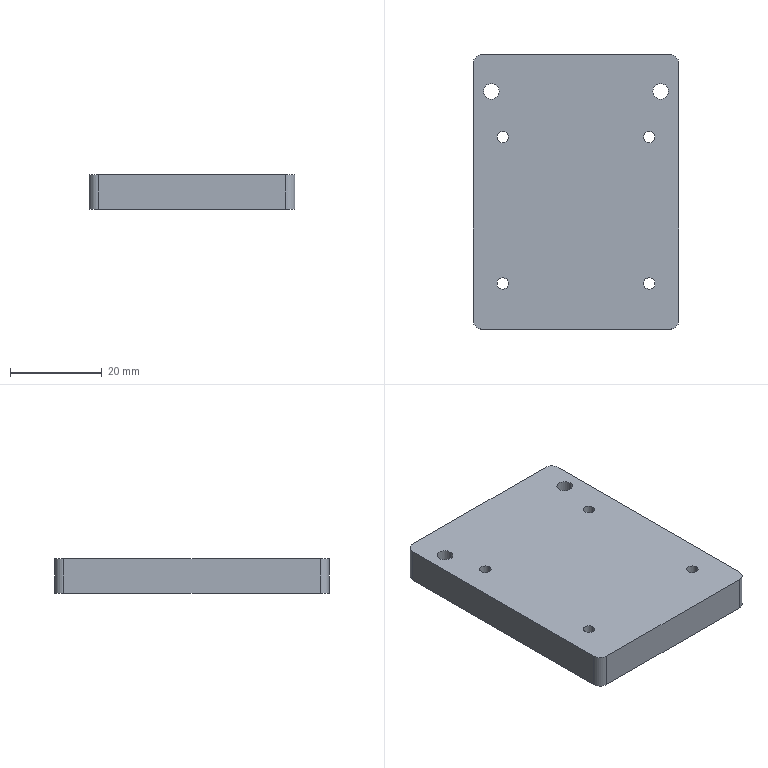Part | STEP file | Guide wheel mechanism revised.sldasm-Part-47 | 1 solid | 28 faces | box 45 x 60 x 7.6 mm | volume 20043 mm3 | cylinder 20 | plane 8 | commonest cylinder face diameters 2.5 x8 3.4 x4 4 x4 6.5 x4
STEP:
#1=CARTESIAN_POINT('',(-15.25,22.,-0.4));
#2=VERTEX_POINT('',#1);
#3=CARTESIAN_POINT('',(-21.75,22.,-0.4));
#4=VERTEX_POINT('',#3);
#5=CARTESIAN_POINT('',(-18.5,22.,-0.4));
#6=DIRECTION('',(0.,0.,-1.));
#7=DIRECTION('',(-1.,0.,0.));
#8=AXIS2_PLACEMENT_3D('',#5,#6,#7);
#9=CIRCLE('',#8,3.25);
#10=EDGE_CURVE('',#2,#4,#9,.T.);
#11=ORIENTED_EDGE('',*,*,#10,.F.);
#12=CARTESIAN_POINT('',(-15.25,22.,-3.8));
#13=VERTEX_POINT('',#12);
#14=CARTESIAN_POINT('',(-15.25,22.,-3.8));
#15=DIRECTION('',(0.,0.,-1.));
#16=VECTOR('',#15,1000.);
#17=LINE('',#14,#16);
#18=EDGE_CURVE('',#2,#13,#17,.T.);
#19=ORIENTED_EDGE('',*,*,#18,.T.);
#20=CARTESIAN_POINT('',(-21.75,22.,-3.8));
#21=VERTEX_POINT('',#20);
#22=CARTESIAN_POINT('',(-18.5,22.,-3.8));
#23=DIRECTION('',(0.,0.,-1.));
#24=DIRECTION('',(-1.,0.,0.));
#25=AXIS2_PLACEMENT_3D('',#22,#23,#24);
#26=CIRCLE('',#25,3.25);
#27=EDGE_CURVE('',#13,#21,#26,.T.);
#28=ORIENTED_EDGE('',*,*,#27,.T.);
#29=CARTESIAN_POINT('',(-21.75,22.,-3.8));
#30=DIRECTION('',(0.,0.,-1.));
#31=VECTOR('',#30,1000.);
#32=LINE('',#29,#31);
#33=EDGE_CURVE('',#4,#21,#32,.T.);
#34=ORIENTED_EDGE('',*,*,#33,.F.);
#35=EDGE_LOOP('',(#11,#19,#28,#34));
#36=FACE_OUTER_BOUND('',#35,.T.);
#37=CARTESIAN_POINT('',(-18.5,22.,-3.8));
#38=DIRECTION('',(0.,0.,-1.));
#39=DIRECTION('',(-1.,0.,0.));
#40=AXIS2_PLACEMENT_3D('',#37,#38,#39);
#41=CYLINDRICAL_SURFACE('',#40,3.25);
#42=ADVANCED_FACE('',(#36),#41,.F.);
#43=CARTESIAN_POINT('',(-16.8,22.,3.8));
#44=VERTEX_POINT('',#43);
#45=CARTESIAN_POINT('',(-20.2,22.,3.8));
#46=VERTEX_POINT('',#45);
#47=CARTESIAN_POINT('',(-18.5,22.,3.8));
#48=DIRECTION('',(0.,0.,-1.));
#49=DIRECTION('',(-1.,0.,0.));
#50=AXIS2_PLACEMENT_3D('',#47,#48,#49);
#51=CIRCLE('',#50,1.7);
#52=EDGE_CURVE('',#44,#46,#51,.T.);
#53=ORIENTED_EDGE('',*,*,#52,.F.);
#54=CARTESIAN_POINT('',(-16.8,22.,-0.4));
#55=VERTEX_POINT('',#54);
#56=CARTESIAN_POINT('',(-16.8,22.,-3.8));
#57=DIRECTION('',(0.,0.,-1.));
#58=VECTOR('',#57,1000.);
#59=LINE('',#56,#58);
#60=EDGE_CURVE('',#44,#55,#59,.T.);
#61=ORIENTED_EDGE('',*,*,#60,.T.);
#62=CARTESIAN_POINT('',(-20.2,22.,-0.4));
#63=VERTEX_POINT('',#62);
#64=CARTESIAN_POINT('',(-18.5,22.,-0.4));
#65=DIRECTION('',(0.,0.,-1.));
#66=DIRECTION('',(-1.,0.,0.));
#67=AXIS2_PLACEMENT_3D('',#64,#65,#66);
#68=CIRCLE('',#67,1.7);
#69=EDGE_CURVE('',#55,#63,#68,.T.);
#70=ORIENTED_EDGE('',*,*,#69,.T.);
#71=CARTESIAN_POINT('',(-20.2,22.,-3.8));
#72=DIRECTION('',(0.,0.,-1.));
#73=VECTOR('',#72,1000.);
#74=LINE('',#71,#73);
#75=EDGE_CURVE('',#46,#63,#74,.T.);
#76=ORIENTED_EDGE('',*,*,#75,.F.);
#77=EDGE_LOOP('',(#53,#61,#70,#76));
#78=FACE_OUTER_BOUND('',#77,.T.);
#79=CARTESIAN_POINT('',(-18.5,22.,-3.8));
#80=DIRECTION('',(0.,0.,-1.));
#81=DIRECTION('',(-1.,0.,0.));
#82=AXIS2_PLACEMENT_3D('',#79,#80,#81);
#83=CYLINDRICAL_SURFACE('',#82,1.7);
#84=ADVANCED_FACE('',(#78),#83,.F.);
#85=CARTESIAN_POINT('',(21.75,22.,-0.4));
#86=VERTEX_POINT('',#85);
#87=CARTESIAN_POINT('',(15.25,22.,-0.4));
#88=VERTEX_POINT('',#87);
#89=CARTESIAN_POINT('',(18.5,22.,-0.4));
#90=DIRECTION('',(0.,0.,-1.));
#91=DIRECTION('',(-1.,0.,0.));
#92=AXIS2_PLACEMENT_3D('',#89,#90,#91);
#93=CIRCLE('',#92,3.25);
#94=EDGE_CURVE('',#86,#88,#93,.T.);
#95=ORIENTED_EDGE('',*,*,#94,.F.);
#96=CARTESIAN_POINT('',(21.75,22.,-3.8));
#97=VERTEX_POINT('',#96);
#98=CARTESIAN_POINT('',(21.75,22.,-3.8));
#99=DIRECTION('',(0.,0.,-1.));
#100=VECTOR('',#99,1000.);
#101=LINE('',#98,#100);
#102=EDGE_CURVE('',#86,#97,#101,.T.);
#103=ORIENTED_EDGE('',*,*,#102,.T.);
#104=CARTESIAN_POINT('',(15.25,22.,-3.8));
#105=VERTEX_POINT('',#104);
#106=CARTESIAN_POINT('',(18.5,22.,-3.8));
#107=DIRECTION('',(0.,0.,-1.));
#108=DIRECTION('',(-1.,0.,0.));
#109=AXIS2_PLACEMENT_3D('',#106,#107,#108);
#110=CIRCLE('',#109,3.25);
#111=EDGE_CURVE('',#97,#105,#110,.T.);
#112=ORIENTED_EDGE('',*,*,#111,.T.);
#113=CARTESIAN_POINT('',(15.25,22.,-3.8));
#114=DIRECTION('',(0.,0.,-1.));
#115=VECTOR('',#114,1000.);
#116=LINE('',#113,#115);
#117=EDGE_CURVE('',#88,#105,#116,.T.);
#118=ORIENTED_EDGE('',*,*,#117,.F.);
#119=EDGE_LOOP('',(#95,#103,#112,#118));
#120=FACE_OUTER_BOUND('',#119,.T.);
#121=CARTESIAN_POINT('',(18.5,22.,-3.8));
#122=DIRECTION('',(0.,0.,-1.));
#123=DIRECTION('',(-1.,0.,0.));
#124=AXIS2_PLACEMENT_3D('',#121,#122,#123);
#125=CYLINDRICAL_SURFACE('',#124,3.25);
#126=ADVANCED_FACE('',(#120),#125,.F.);
#127=CARTESIAN_POINT('',(20.2,22.,3.8));
#128=VERTEX_POINT('',#127);
#129=CARTESIAN_POINT('',(16.8,22.,3.8));
#130=VERTEX_POINT('',#129);
#131=CARTESIAN_POINT('',(18.5,22.,3.8));
#132=DIRECTION('',(0.,0.,-1.));
#133=DIRECTION('',(-1.,0.,0.));
#134=AXIS2_PLACEMENT_3D('',#131,#132,#133);
#135=CIRCLE('',#134,1.7);
#136=EDGE_CURVE('',#128,#130,#135,.T.);
#137=ORIENTED_EDGE('',*,*,#136,.F.);
#138=CARTESIAN_POINT('',(20.2,22.,-0.4));
#139=VERTEX_POINT('',#138);
#140=CARTESIAN_POINT('',(20.2,22.,-3.8));
#141=DIRECTION('',(0.,0.,-1.));
#142=VECTOR('',#141,1000.);
#143=LINE('',#140,#142);
#144=EDGE_CURVE('',#128,#139,#143,.T.);
#145=ORIENTED_EDGE('',*,*,#144,.T.);
#146=CARTESIAN_POINT('',(16.8,22.,-0.4));
#147=VERTEX_POINT('',#146);
#148=CARTESIAN_POINT('',(18.5,22.,-0.4));
#149=DIRECTION('',(0.,0.,-1.));
#150=DIRECTION('',(-1.,0.,0.));
#151=AXIS2_PLACEMENT_3D('',#148,#149,#150);
#152=CIRCLE('',#151,1.7);
#153=EDGE_CURVE('',#139,#147,#152,.T.);
#154=ORIENTED_EDGE('',*,*,#153,.T.);
#155=CARTESIAN_POINT('',(16.8,22.,-3.8));
#156=DIRECTION('',(0.,0.,-1.));
#157=VECTOR('',#156,1000.);
#158=LINE('',#155,#157);
#159=EDGE_CURVE('',#130,#147,#158,.T.);
#160=ORIENTED_EDGE('',*,*,#159,.F.);
#161=EDGE_LOOP('',(#137,#145,#154,#160));
#162=FACE_OUTER_BOUND('',#161,.T.);
#163=CARTESIAN_POINT('',(18.5,22.,-3.8));
#164=DIRECTION('',(0.,0.,-1.));
#165=DIRECTION('',(-1.,0.,0.));
#166=AXIS2_PLACEMENT_3D('',#163,#164,#165);
#167=CYLINDRICAL_SURFACE('',#166,1.7);
#168=ADVANCED_FACE('',(#162),#167,.F.);
#169=CARTESIAN_POINT('',(14.75,12.,-3.8));
#170=VERTEX_POINT('',#169);
#171=CARTESIAN_POINT('',(17.25,12.,-3.8));
#172=VERTEX_POINT('',#171);
#173=CARTESIAN_POINT('',(16.,12.,-3.8));
#174=DIRECTION('',(0.,0.,1.));
#175=DIRECTION('',(1.,0.,0.));
#176=AXIS2_PLACEMENT_3D('',#173,#174,#175);
#177=CIRCLE('',#176,1.25);
#178=EDGE_CURVE('',#170,#172,#177,.T.);
#179=ORIENTED_EDGE('',*,*,#178,.F.);
#180=CARTESIAN_POINT('',(14.75,12.,3.8));
#181=VERTEX_POINT('',#180);
#182=CARTESIAN_POINT('',(14.75,12.,3.8));
#183=DIRECTION('',(0.,0.,1.));
#184=VECTOR('',#183,1000.);
#185=LINE('',#182,#184);
#186=EDGE_CURVE('',#170,#181,#185,.T.);
#187=ORIENTED_EDGE('',*,*,#186,.T.);
#188=CARTESIAN_POINT('',(17.25,12.,3.8));
#189=VERTEX_POINT('',#188);
#190=CARTESIAN_POINT('',(16.,12.,3.8));
#191=DIRECTION('',(0.,0.,1.));
#192=DIRECTION('',(1.,0.,0.));
#193=AXIS2_PLACEMENT_3D('',#190,#191,#192);
#194=CIRCLE('',#193,1.25);
#195=EDGE_CURVE('',#181,#189,#194,.T.);
#196=ORIENTED_EDGE('',*,*,#195,.T.);
#197=CARTESIAN_POINT('',(17.25,12.,3.8));
#198=DIRECTION('',(0.,0.,1.));
#199=VECTOR('',#198,1000.);
#200=LINE('',#197,#199);
#201=EDGE_CURVE('',#172,#189,#200,.T.);
#202=ORIENTED_EDGE('',*,*,#201,.F.);
#203=EDGE_LOOP('',(#179,#187,#196,#202));
#204=FACE_OUTER_BOUND('',#203,.T.);
#205=CARTESIAN_POINT('',(16.,12.,3.8));
#206=DIRECTION('',(0.,0.,1.));
#207=DIRECTION('',(1.,0.,0.));
#208=AXIS2_PLACEMENT_3D('',#205,#206,#207);
#209=CYLINDRICAL_SURFACE('',#208,1.25);
#210=ADVANCED_FACE('',(#204),#209,.F.);
#211=CARTESIAN_POINT('',(-17.25,12.,-3.8));
#212=VERTEX_POINT('',#211);
#213=CARTESIAN_POINT('',(-14.75,12.,-3.8));
#214=VERTEX_POINT('',#213);
#215=CARTESIAN_POINT('',(-16.,12.,-3.8));
#216=DIRECTION('',(0.,0.,1.));
#217=DIRECTION('',(1.,0.,0.));
#218=AXIS2_PLACEMENT_3D('',#215,#216,#217);
#219=CIRCLE('',#218,1.25);
#220=EDGE_CURVE('',#212,#214,#219,.T.);
#221=ORIENTED_EDGE('',*,*,#220,.F.);
#222=CARTESIAN_POINT('',(-17.25,12.,3.8));
#223=VERTEX_POINT('',#222);
#224=CARTESIAN_POINT('',(-17.25,12.,3.8));
#225=DIRECTION('',(0.,0.,1.));
#226=VECTOR('',#225,1000.);
#227=LINE('',#224,#226);
#228=EDGE_CURVE('',#212,#223,#227,.T.);
#229=ORIENTED_EDGE('',*,*,#228,.T.);
#230=CARTESIAN_POINT('',(-14.75,12.,3.8));
#231=VERTEX_POINT('',#230);
#232=CARTESIAN_POINT('',(-16.,12.,3.8));
#233=DIRECTION('',(0.,0.,1.));
#234=DIRECTION('',(1.,0.,0.));
#235=AXIS2_PLACEMENT_3D('',#232,#233,#234);
#236=CIRCLE('',#235,1.25);
#237=EDGE_CURVE('',#223,#231,#236,.T.);
#238=ORIENTED_EDGE('',*,*,#237,.T.);
#239=CARTESIAN_POINT('',(-14.75,12.,3.8));
#240=DIRECTION('',(0.,0.,1.));
#241=VECTOR('',#240,1000.);
#242=LINE('',#239,#241);
#243=EDGE_CURVE('',#214,#231,#242,.T.);
#244=ORIENTED_EDGE('',*,*,#243,.F.);
#245=EDGE_LOOP('',(#221,#229,#238,#244));
#246=FACE_OUTER_BOUND('',#245,.T.);
#247=CARTESIAN_POINT('',(-16.,12.,3.8));
#248=DIRECTION('',(0.,0.,1.));
#249=DIRECTION('',(1.,0.,0.));
#250=AXIS2_PLACEMENT_3D('',#247,#248,#249);
#251=CYLINDRICAL_SURFACE('',#250,1.25);
#252=ADVANCED_FACE('',(#246),#251,.F.);
#253=CARTESIAN_POINT('',(-17.25,-20.,-3.8));
#254=VERTEX_POINT('',#253);
#255=CARTESIAN_POINT('',(-14.75,-20.,-3.8));
#256=VERTEX_POINT('',#255);
#257=CARTESIAN_POINT('',(-16.,-20.,-3.8));
#258=DIRECTION('',(0.,0.,1.));
#259=DIRECTION('',(1.,0.,0.));
#260=AXIS2_PLACEMENT_3D('',#257,#258,#259);
#261=CIRCLE('',#260,1.25);
#262=EDGE_CURVE('',#254,#256,#261,.T.);
#263=ORIENTED_EDGE('',*,*,#262,.F.);
#264=CARTESIAN_POINT('',(-17.25,-20.,3.8));
#265=VERTEX_POINT('',#264);
#266=CARTESIAN_POINT('',(-17.25,-20.,3.8));
#267=DIRECTION('',(0.,0.,1.));
#268=VECTOR('',#267,1000.);
#269=LINE('',#266,#268);
#270=EDGE_CURVE('',#254,#265,#269,.T.);
#271=ORIENTED_EDGE('',*,*,#270,.T.);
#272=CARTESIAN_POINT('',(-14.75,-20.,3.8));
#273=VERTEX_POINT('',#272);
#274=CARTESIAN_POINT('',(-16.,-20.,3.8));
#275=DIRECTION('',(0.,0.,1.));
#276=DIRECTION('',(1.,0.,0.));
#277=AXIS2_PLACEMENT_3D('',#274,#275,#276);
#278=CIRCLE('',#277,1.25);
#279=EDGE_CURVE('',#265,#273,#278,.T.);
#280=ORIENTED_EDGE('',*,*,#279,.T.);
#281=CARTESIAN_POINT('',(-14.75,-20.,3.8));
#282=DIRECTION('',(0.,0.,1.));
#283=VECTOR('',#282,1000.);
#284=LINE('',#281,#283);
#285=EDGE_CURVE('',#256,#273,#284,.T.);
#286=ORIENTED_EDGE('',*,*,#285,.F.);
#287=EDGE_LOOP('',(#263,#271,#280,#286));
#288=FACE_OUTER_BOUND('',#287,.T.);
#289=CARTESIAN_POINT('',(-16.,-20.,3.8));
#290=DIRECTION('',(0.,0.,1.));
#291=DIRECTION('',(1.,0.,0.));
#292=AXIS2_PLACEMENT_3D('',#289,#290,#291);
#293=CYLINDRICAL_SURFACE('',#292,1.25);
#294=ADVANCED_FACE('',(#288),#293,.F.);
#295=CARTESIAN_POINT('',(14.75,-20.,-3.8));
#296=VERTEX_POINT('',#295);
#297=CARTESIAN_POINT('',(17.25,-20.,-3.8));
#298=VERTEX_POINT('',#297);
#299=CARTESIAN_POINT('',(16.,-20.,-3.8));
#300=DIRECTION('',(0.,0.,1.));
#301=DIRECTION('',(1.,0.,0.));
#302=AXIS2_PLACEMENT_3D('',#299,#300,#301);
#303=CIRCLE('',#302,1.25);
#304=EDGE_CURVE('',#296,#298,#303,.T.);
#305=ORIENTED_EDGE('',*,*,#304,.F.);
#306=CARTESIAN_POINT('',(14.75,-20.,3.8));
#307=VERTEX_POINT('',#306);
#308=CARTESIAN_POINT('',(14.75,-20.,3.8));
#309=DIRECTION('',(0.,0.,1.));
#310=VECTOR('',#309,1000.);
#311=LINE('',#308,#310);
#312=EDGE_CURVE('',#296,#307,#311,.T.);
#313=ORIENTED_EDGE('',*,*,#312,.T.);
#314=CARTESIAN_POINT('',(17.25,-20.,3.8));
#315=VERTEX_POINT('',#314);
#316=CARTESIAN_POINT('',(16.,-20.,3.8));
#317=DIRECTION('',(0.,0.,1.));
#318=DIRECTION('',(1.,0.,0.));
#319=AXIS2_PLACEMENT_3D('',#316,#317,#318);
#320=CIRCLE('',#319,1.25);
#321=EDGE_CURVE('',#307,#315,#320,.T.);
#322=ORIENTED_EDGE('',*,*,#321,.T.);
#323=CARTESIAN_POINT('',(17.25,-20.,3.8));
#324=DIRECTION('',(0.,0.,1.));
#325=VECTOR('',#324,1000.);
#326=LINE('',#323,#325);
#327=EDGE_CURVE('',#298,#315,#326,.T.);
#328=ORIENTED_EDGE('',*,*,#327,.F.);
#329=EDGE_LOOP('',(#305,#313,#322,#328));
#330=FACE_OUTER_BOUND('',#329,.T.);
#331=CARTESIAN_POINT('',(16.,-20.,3.8));
#332=DIRECTION('',(0.,0.,1.));
#333=DIRECTION('',(1.,0.,0.));
#334=AXIS2_PLACEMENT_3D('',#331,#332,#333);
#335=CYLINDRICAL_SURFACE('',#334,1.25);
#336=ADVANCED_FACE('',(#330),#335,.F.);
#337=CARTESIAN_POINT('',(22.5,-28.,3.8));
#338=VERTEX_POINT('',#337);
#339=CARTESIAN_POINT('',(22.5,28.,3.8));
#340=VERTEX_POINT('',#339);
#341=CARTESIAN_POINT('',(22.5,-30.,3.8));
#342=DIRECTION('',(0.,1.,0.));
#343=VECTOR('',#342,1000.);
#344=LINE('',#341,#343);
#345=EDGE_CURVE('',#338,#340,#344,.T.);
#346=ORIENTED_EDGE('',*,*,#345,.F.);
#347=CARTESIAN_POINT('',(22.5,-28.,-3.8));
#348=VERTEX_POINT('',#347);
#349=CARTESIAN_POINT('',(22.5,-28.,3.8));
#350=DIRECTION('',(0.,0.,-1.));
#351=VECTOR('',#350,1000.);
#352=LINE('',#349,#351);
#353=EDGE_CURVE('',#338,#348,#352,.T.);
#354=ORIENTED_EDGE('',*,*,#353,.T.);
#355=CARTESIAN_POINT('',(22.5,28.,-3.8));
#356=VERTEX_POINT('',#355);
#357=CARTESIAN_POINT('',(22.5,-30.,-3.8));
#358=DIRECTION('',(0.,1.,0.));
#359=VECTOR('',#358,1000.);
#360=LINE('',#357,#359);
#361=EDGE_CURVE('',#348,#356,#360,.T.);
#362=ORIENTED_EDGE('',*,*,#361,.T.);
#363=CARTESIAN_POINT('',(22.5,28.,3.8));
#364=DIRECTION('',(0.,0.,1.));
#365=VECTOR('',#364,1000.);
#366=LINE('',#363,#365);
#367=EDGE_CURVE('',#356,#340,#366,.T.);
#368=ORIENTED_EDGE('',*,*,#367,.T.);
#369=EDGE_LOOP('',(#346,#354,#362,#368));
#370=FACE_OUTER_BOUND('',#369,.T.);
#371=CARTESIAN_POINT('',(22.5,-30.,3.8));
#372=DIRECTION('',(-1.,0.,0.));
#373=DIRECTION('',(0.,0.,1.));
#374=AXIS2_PLACEMENT_3D('',#371,#372,#373);
#375=PLANE('',#374);
#376=ADVANCED_FACE('',(#370),#375,.F.);
#377=CARTESIAN_POINT('',(20.5,30.,-3.8));
#378=VERTEX_POINT('',#377);
#379=CARTESIAN_POINT('',(-20.5,30.,-3.8));
#380=VERTEX_POINT('',#379);
#381=CARTESIAN_POINT('',(-22.5,30.,-3.8));
#382=DIRECTION('',(-1.,0.,0.));
#383=VECTOR('',#382,1000.);
#384=LINE('',#381,#383);
#385=EDGE_CURVE('',#378,#380,#384,.T.);
#386=ORIENTED_EDGE('',*,*,#385,.T.);
#387=CARTESIAN_POINT('',(-20.5,30.,3.8));
#388=VERTEX_POINT('',#387);
#389=CARTESIAN_POINT('',(-20.5,30.,3.8));
#390=DIRECTION('',(0.,0.,1.));
#391=VECTOR('',#390,1000.);
#392=LINE('',#389,#391);
#393=EDGE_CURVE('',#380,#388,#392,.T.);
#394=ORIENTED_EDGE('',*,*,#393,.T.);
#395=CARTESIAN_POINT('',(20.5,30.,3.8));
#396=VERTEX_POINT('',#395);
#397=CARTESIAN_POINT('',(-22.5,30.,3.8));
#398=DIRECTION('',(-1.,0.,0.));
#399=VECTOR('',#398,1000.);
#400=LINE('',#397,#399);
#401=EDGE_CURVE('',#396,#388,#400,.T.);
#402=ORIENTED_EDGE('',*,*,#401,.F.);
#403=CARTESIAN_POINT('',(20.5,30.,3.8));
#404=DIRECTION('',(0.,0.,-1.));
#405=VECTOR('',#404,1000.);
#406=LINE('',#403,#405);
#407=EDGE_CURVE('',#396,#378,#406,.T.);
#408=ORIENTED_EDGE('',*,*,#407,.T.);
#409=EDGE_LOOP('',(#386,#394,#402,#408));
#410=FACE_OUTER_BOUND('',#409,.T.);
#411=CARTESIAN_POINT('',(-22.5,30.,3.8));
#412=DIRECTION('',(0.,-1.,0.));
#413=DIRECTION('',(0.,0.,-1.));
#414=AXIS2_PLACEMENT_3D('',#411,#412,#413);
#415=PLANE('',#414);
#416=ADVANCED_FACE('',(#410),#415,.F.);
#417=CARTESIAN_POINT('',(-22.5,28.,-3.8));
#418=VERTEX_POINT('',#417);
#419=CARTESIAN_POINT('',(-22.5,-28.,-3.8));
#420=VERTEX_POINT('',#419);
#421=CARTESIAN_POINT('',(-22.5,-30.,-3.8));
#422=DIRECTION('',(0.,-1.,0.));
#423=VECTOR('',#422,1000.);
#424=LINE('',#421,#423);
#425=EDGE_CURVE('',#418,#420,#424,.T.);
#426=ORIENTED_EDGE('',*,*,#425,.T.);
#427=CARTESIAN_POINT('',(-22.5,-28.,3.8));
#428=VERTEX_POINT('',#427);
#429=CARTESIAN_POINT('',(-22.5,-28.,3.8));
#430=DIRECTION('',(0.,0.,1.));
#431=VECTOR('',#430,1000.);
#432=LINE('',#429,#431);
#433=EDGE_CURVE('',#420,#428,#432,.T.);
#434=ORIENTED_EDGE('',*,*,#433,.T.);
#435=CARTESIAN_POINT('',(-22.5,28.,3.8));
#436=VERTEX_POINT('',#435);
#437=CARTESIAN_POINT('',(-22.5,-30.,3.8));
#438=DIRECTION('',(0.,-1.,0.));
#439=VECTOR('',#438,1000.);
#440=LINE('',#437,#439);
#441=EDGE_CURVE('',#436,#428,#440,.T.);
#442=ORIENTED_EDGE('',*,*,#441,.F.);
#443=CARTESIAN_POINT('',(-22.5,28.,3.8));
#444=DIRECTION('',(0.,0.,-1.));
#445=VECTOR('',#444,1000.);
#446=LINE('',#443,#445);
#447=EDGE_CURVE('',#436,#418,#446,.T.);
#448=ORIENTED_EDGE('',*,*,#447,.T.);
#449=EDGE_LOOP('',(#426,#434,#442,#448));
#450=FACE_OUTER_BOUND('',#449,.T.);
#451=CARTESIAN_POINT('',(-22.5,-30.,3.8));
#452=DIRECTION('',(1.,0.,0.));
#453=DIRECTION('',(0.,0.,-1.));
#454=AXIS2_PLACEMENT_3D('',#451,#452,#453);
#455=PLANE('',#454);
#456=ADVANCED_FACE('',(#450),#455,.F.);
#457=CARTESIAN_POINT('',(-20.5,-30.,3.8));
#458=VERTEX_POINT('',#457);
#459=CARTESIAN_POINT('',(20.5,-30.,3.8));
#460=VERTEX_POINT('',#459);
#461=CARTESIAN_POINT('',(-22.5,-30.,3.8));
#462=DIRECTION('',(1.,0.,0.));
#463=VECTOR('',#462,1000.);
#464=LINE('',#461,#463);
#465=EDGE_CURVE('',#458,#460,#464,.T.);
#466=ORIENTED_EDGE('',*,*,#465,.F.);
#467=CARTESIAN_POINT('',(-20.5,-30.,-3.8));
#468=VERTEX_POINT('',#467);
#469=CARTESIAN_POINT('',(-20.5,-30.,3.8));
#470=DIRECTION('',(0.,0.,-1.));
#471=VECTOR('',#470,1000.);
#472=LINE('',#469,#471);
#473=EDGE_CURVE('',#458,#468,#472,.T.);
#474=ORIENTED_EDGE('',*,*,#473,.T.);
#475=CARTESIAN_POINT('',(20.5,-30.,-3.8));
#476=VERTEX_POINT('',#475);
#477=CARTESIAN_POINT('',(-22.5,-30.,-3.8));
#478=DIRECTION('',(1.,0.,0.));
#479=VECTOR('',#478,1000.);
#480=LINE('',#477,#479);
#481=EDGE_CURVE('',#468,#476,#480,.T.);
#482=ORIENTED_EDGE('',*,*,#481,.T.);
#483=CARTESIAN_POINT('',(20.5,-30.,3.8));
#484=DIRECTION('',(0.,0.,1.));
#485=VECTOR('',#484,1000.);
#486=LINE('',#483,#485);
#487=EDGE_CURVE('',#476,#460,#486,.T.);
#488=ORIENTED_EDGE('',*,*,#487,.T.);
#489=EDGE_LOOP('',(#466,#474,#482,#488));
#490=FACE_OUTER_BOUND('',#489,.T.);
#491=CARTESIAN_POINT('',(-22.5,-30.,3.8));
#492=DIRECTION('',(0.,1.,0.));
#493=DIRECTION('',(0.,0.,1.));
#494=AXIS2_PLACEMENT_3D('',#491,#492,#493);
#495=PLANE('',#494);
#496=ADVANCED_FACE('',(#490),#495,.F.);
#497=CARTESIAN_POINT('',(-18.5,22.,3.8));
#498=DIRECTION('',(0.,0.,-1.));
#499=DIRECTION('',(-1.,0.,0.));
#500=AXIS2_PLACEMENT_3D('',#497,#498,#499);
#501=CIRCLE('',#500,1.7);
#502=EDGE_CURVE('',#46,#44,#501,.T.);
#503=ORIENTED_EDGE('',*,*,#502,.T.);
#504=ORIENTED_EDGE('',*,*,#52,.T.);
#505=EDGE_LOOP('',(#503,#504));
#506=FACE_BOUND('',#505,.T.);
#507=CARTESIAN_POINT('',(18.5,22.,3.8));
#508=DIRECTION('',(0.,0.,-1.));
#509=DIRECTION('',(-1.,0.,0.));
#510=AXIS2_PLACEMENT_3D('',#507,#508,#509);
#511=CIRCLE('',#510,1.7);
#512=EDGE_CURVE('',#130,#128,#511,.T.);
#513=ORIENTED_EDGE('',*,*,#512,.T.);
#514=ORIENTED_EDGE('',*,*,#136,.T.);
#515=EDGE_LOOP('',(#513,#514));
#516=FACE_BOUND('',#515,.T.);
#517=CARTESIAN_POINT('',(16.,12.,3.8));
#518=DIRECTION('',(0.,0.,1.));
#519=DIRECTION('',(1.,0.,0.));
#520=AXIS2_PLACEMENT_3D('',#517,#518,#519);
#521=CIRCLE('',#520,1.25);
#522=EDGE_CURVE('',#189,#181,#521,.T.);
#523=ORIENTED_EDGE('',*,*,#522,.F.);
#524=ORIENTED_EDGE('',*,*,#195,.F.);
#525=EDGE_LOOP('',(#523,#524));
#526=FACE_BOUND('',#525,.T.);
#527=CARTESIAN_POINT('',(-16.,12.,3.8));
#528=DIRECTION('',(0.,0.,1.));
#529=DIRECTION('',(1.,0.,0.));
#530=AXIS2_PLACEMENT_3D('',#527,#528,#529);
#531=CIRCLE('',#530,1.25);
#532=EDGE_CURVE('',#231,#223,#531,.T.);
#533=ORIENTED_EDGE('',*,*,#532,.F.);
#534=ORIENTED_EDGE('',*,*,#237,.F.);
#535=EDGE_LOOP('',(#533,#534));
#536=FACE_BOUND('',#535,.T.);
#537=CARTESIAN_POINT('',(-16.,-20.,3.8));
#538=DIRECTION('',(0.,0.,1.));
#539=DIRECTION('',(1.,0.,0.));
#540=AXIS2_PLACEMENT_3D('',#537,#538,#539);
#541=CIRCLE('',#540,1.25);
#542=EDGE_CURVE('',#273,#265,#541,.T.);
#543=ORIENTED_EDGE('',*,*,#542,.F.);
#544=ORIENTED_EDGE('',*,*,#279,.F.);
#545=EDGE_LOOP('',(#543,#544));
#546=FACE_BOUND('',#545,.T.);
#547=CARTESIAN_POINT('',(16.,-20.,3.8));
#548=DIRECTION('',(0.,0.,1.));
#549=DIRECTION('',(1.,0.,0.));
#550=AXIS2_PLACEMENT_3D('',#547,#548,#549);
#551=CIRCLE('',#550,1.25);
#552=EDGE_CURVE('',#315,#307,#551,.T.);
#553=ORIENTED_EDGE('',*,*,#552,.F.);
#554=ORIENTED_EDGE('',*,*,#321,.F.);
#555=EDGE_LOOP('',(#553,#554));
#556=FACE_BOUND('',#555,.T.);
#557=ORIENTED_EDGE('',*,*,#441,.T.);
#558=CARTESIAN_POINT('',(-20.5,-28.,3.8));
#559=DIRECTION('',(0.,0.,1.));
#560=DIRECTION('',(-1.,0.,0.));
#561=AXIS2_PLACEMENT_3D('',#558,#559,#560);
#562=CIRCLE('',#561,2.);
#563=EDGE_CURVE('',#428,#458,#562,.T.);
#564=ORIENTED_EDGE('',*,*,#563,.T.);
#565=ORIENTED_EDGE('',*,*,#465,.T.);
#566=CARTESIAN_POINT('',(20.5,-28.,3.8));
#567=DIRECTION('',(0.,0.,1.));
#568=DIRECTION('',(-1.,0.,0.));
#569=AXIS2_PLACEMENT_3D('',#566,#567,#568);
#570=CIRCLE('',#569,2.);
#571=EDGE_CURVE('',#460,#338,#570,.T.);
#572=ORIENTED_EDGE('',*,*,#571,.T.);
#573=ORIENTED_EDGE('',*,*,#345,.T.);
#574=CARTESIAN_POINT('',(20.5,28.,3.8));
#575=DIRECTION('',(0.,0.,1.));
#576=DIRECTION('',(-1.,0.,0.));
#577=AXIS2_PLACEMENT_3D('',#574,#575,#576);
#578=CIRCLE('',#577,2.);
#579=EDGE_CURVE('',#340,#396,#578,.T.);
#580=ORIENTED_EDGE('',*,*,#579,.T.);
#581=ORIENTED_EDGE('',*,*,#401,.T.);
#582=CARTESIAN_POINT('',(-20.5,28.,3.8));
#583=DIRECTION('',(0.,0.,1.));
#584=DIRECTION('',(-1.,0.,0.));
#585=AXIS2_PLACEMENT_3D('',#582,#583,#584);
#586=CIRCLE('',#585,2.);
#587=EDGE_CURVE('',#388,#436,#586,.T.);
#588=ORIENTED_EDGE('',*,*,#587,.T.);
#589=EDGE_LOOP('',(#557,#564,#565,#572,#573,#580,#581,#588));
#590=FACE_OUTER_BOUND('',#589,.T.);
#591=CARTESIAN_POINT('',(0.,0.,3.8));
#592=DIRECTION('',(0.,0.,-1.));
#593=DIRECTION('',(-1.,0.,0.));
#594=AXIS2_PLACEMENT_3D('',#591,#592,#593);
#595=PLANE('',#594);
#596=ADVANCED_FACE('',(#506,#516,#526,#536,#546,#556,#590),#595,.F.);
#597=CARTESIAN_POINT('',(-18.5,22.,-3.8));
#598=DIRECTION('',(0.,0.,-1.));
#599=DIRECTION('',(-1.,0.,0.));
#600=AXIS2_PLACEMENT_3D('',#597,#598,#599);
#601=CIRCLE('',#600,3.25);
#602=EDGE_CURVE('',#21,#13,#601,.T.);
#603=ORIENTED_EDGE('',*,*,#602,.F.);
#604=ORIENTED_EDGE('',*,*,#27,.F.);
#605=EDGE_LOOP('',(#603,#604));
#606=FACE_BOUND('',#605,.T.);
#607=CARTESIAN_POINT('',(18.5,22.,-3.8));
#608=DIRECTION('',(0.,0.,-1.));
#609=DIRECTION('',(-1.,0.,0.));
#610=AXIS2_PLACEMENT_3D('',#607,#608,#609);
#611=CIRCLE('',#610,3.25);
#612=EDGE_CURVE('',#105,#97,#611,.T.);
#613=ORIENTED_EDGE('',*,*,#612,.F.);
#614=ORIENTED_EDGE('',*,*,#111,.F.);
#615=EDGE_LOOP('',(#613,#614));
#616=FACE_BOUND('',#615,.T.);
#617=CARTESIAN_POINT('',(16.,12.,-3.8));
#618=DIRECTION('',(0.,0.,1.));
#619=DIRECTION('',(1.,0.,0.));
#620=AXIS2_PLACEMENT_3D('',#617,#618,#619);
#621=CIRCLE('',#620,1.25);
#622=EDGE_CURVE('',#172,#170,#621,.T.);
#623=ORIENTED_EDGE('',*,*,#622,.T.);
#624=ORIENTED_EDGE('',*,*,#178,.T.);
#625=EDGE_LOOP('',(#623,#624));
#626=FACE_BOUND('',#625,.T.);
#627=CARTESIAN_POINT('',(-16.,12.,-3.8));
#628=DIRECTION('',(0.,0.,1.));
#629=DIRECTION('',(1.,0.,0.));
#630=AXIS2_PLACEMENT_3D('',#627,#628,#629);
#631=CIRCLE('',#630,1.25);
#632=EDGE_CURVE('',#214,#212,#631,.T.);
#633=ORIENTED_EDGE('',*,*,#632,.T.);
#634=ORIENTED_EDGE('',*,*,#220,.T.);
#635=EDGE_LOOP('',(#633,#634));
#636=FACE_BOUND('',#635,.T.);
#637=CARTESIAN_POINT('',(-16.,-20.,-3.8));
#638=DIRECTION('',(0.,0.,1.));
#639=DIRECTION('',(1.,0.,0.));
#640=AXIS2_PLACEMENT_3D('',#637,#638,#639);
#641=CIRCLE('',#640,1.25);
#642=EDGE_CURVE('',#256,#254,#641,.T.);
#643=ORIENTED_EDGE('',*,*,#642,.T.);
#644=ORIENTED_EDGE('',*,*,#262,.T.);
#645=EDGE_LOOP('',(#643,#644));
#646=FACE_BOUND('',#645,.T.);
#647=CARTESIAN_POINT('',(16.,-20.,-3.8));
#648=DIRECTION('',(0.,0.,1.));
#649=DIRECTION('',(1.,0.,0.));
#650=AXIS2_PLACEMENT_3D('',#647,#648,#649);
#651=CIRCLE('',#650,1.25);
#652=EDGE_CURVE('',#298,#296,#651,.T.);
#653=ORIENTED_EDGE('',*,*,#652,.T.);
#654=ORIENTED_EDGE('',*,*,#304,.T.);
#655=EDGE_LOOP('',(#653,#654));
#656=FACE_BOUND('',#655,.T.);
#657=ORIENTED_EDGE('',*,*,#481,.F.);
#658=CARTESIAN_POINT('',(-20.5,-28.,-3.8));
#659=DIRECTION('',(0.,0.,-1.));
#660=DIRECTION('',(-1.,0.,0.));
#661=AXIS2_PLACEMENT_3D('',#658,#659,#660);
#662=CIRCLE('',#661,2.);
#663=EDGE_CURVE('',#468,#420,#662,.T.);
#664=ORIENTED_EDGE('',*,*,#663,.T.);
#665=ORIENTED_EDGE('',*,*,#425,.F.);
#666=CARTESIAN_POINT('',(-20.5,28.,-3.8));
#667=DIRECTION('',(0.,0.,-1.));
#668=DIRECTION('',(-1.,0.,0.));
#669=AXIS2_PLACEMENT_3D('',#666,#667,#668);
#670=CIRCLE('',#669,2.);
#671=EDGE_CURVE('',#418,#380,#670,.T.);
#672=ORIENTED_EDGE('',*,*,#671,.T.);
#673=ORIENTED_EDGE('',*,*,#385,.F.);
#674=CARTESIAN_POINT('',(20.5,28.,-3.8));
#675=DIRECTION('',(0.,0.,-1.));
#676=DIRECTION('',(-1.,0.,0.));
#677=AXIS2_PLACEMENT_3D('',#674,#675,#676);
#678=CIRCLE('',#677,2.);
#679=EDGE_CURVE('',#378,#356,#678,.T.);
#680=ORIENTED_EDGE('',*,*,#679,.T.);
#681=ORIENTED_EDGE('',*,*,#361,.F.);
#682=CARTESIAN_POINT('',(20.5,-28.,-3.8));
#683=DIRECTION('',(0.,0.,-1.));
#684=DIRECTION('',(-1.,0.,0.));
#685=AXIS2_PLACEMENT_3D('',#682,#683,#684);
#686=CIRCLE('',#685,2.);
#687=EDGE_CURVE('',#348,#476,#686,.T.);
#688=ORIENTED_EDGE('',*,*,#687,.T.);
#689=EDGE_LOOP('',(#657,#664,#665,#672,#673,#680,#681,#688));
#690=FACE_OUTER_BOUND('',#689,.T.);
#691=CARTESIAN_POINT('',(0.,0.,-3.8));
#692=DIRECTION('',(0.,0.,-1.));
#693=DIRECTION('',(-1.,0.,0.));
#694=AXIS2_PLACEMENT_3D('',#691,#692,#693);
#695=PLANE('',#694);
#696=ADVANCED_FACE('',(#606,#616,#626,#636,#646,#656,#690),#695,.T.);
#697=ORIENTED_EDGE('',*,*,#312,.F.);
#698=ORIENTED_EDGE('',*,*,#652,.F.);
#699=ORIENTED_EDGE('',*,*,#327,.T.);
#700=ORIENTED_EDGE('',*,*,#552,.T.);
#701=EDGE_LOOP('',(#697,#698,#699,#700));
#702=FACE_OUTER_BOUND('',#701,.T.);
#703=CARTESIAN_POINT('',(16.,-20.,3.8));
#704=DIRECTION('',(0.,0.,1.));
#705=DIRECTION('',(1.,0.,0.));
#706=AXIS2_PLACEMENT_3D('',#703,#704,#705);
#707=CYLINDRICAL_SURFACE('',#706,1.25);
#708=ADVANCED_FACE('',(#702),#707,.F.);
#709=ORIENTED_EDGE('',*,*,#270,.F.);
#710=ORIENTED_EDGE('',*,*,#642,.F.);
#711=ORIENTED_EDGE('',*,*,#285,.T.);
#712=ORIENTED_EDGE('',*,*,#542,.T.);
#713=EDGE_LOOP('',(#709,#710,#711,#712));
#714=FACE_OUTER_BOUND('',#713,.T.);
#715=CARTESIAN_POINT('',(-16.,-20.,3.8));
#716=DIRECTION('',(0.,0.,1.));
#717=DIRECTION('',(1.,0.,0.));
#718=AXIS2_PLACEMENT_3D('',#715,#716,#717);
#719=CYLINDRICAL_SURFACE('',#718,1.25);
#720=ADVANCED_FACE('',(#714),#719,.F.);
#721=ORIENTED_EDGE('',*,*,#228,.F.);
#722=ORIENTED_EDGE('',*,*,#632,.F.);
#723=ORIENTED_EDGE('',*,*,#243,.T.);
#724=ORIENTED_EDGE('',*,*,#532,.T.);
#725=EDGE_LOOP('',(#721,#722,#723,#724));
#726=FACE_OUTER_BOUND('',#725,.T.);
#727=CARTESIAN_POINT('',(-16.,12.,3.8));
#728=DIRECTION('',(0.,0.,1.));
#729=DIRECTION('',(1.,0.,0.));
#730=AXIS2_PLACEMENT_3D('',#727,#728,#729);
#731=CYLINDRICAL_SURFACE('',#730,1.25);
#732=ADVANCED_FACE('',(#726),#731,.F.);
#733=ORIENTED_EDGE('',*,*,#186,.F.);
#734=ORIENTED_EDGE('',*,*,#622,.F.);
#735=ORIENTED_EDGE('',*,*,#201,.T.);
#736=ORIENTED_EDGE('',*,*,#522,.T.);
#737=EDGE_LOOP('',(#733,#734,#735,#736));
#738=FACE_OUTER_BOUND('',#737,.T.);
#739=CARTESIAN_POINT('',(16.,12.,3.8));
#740=DIRECTION('',(0.,0.,1.));
#741=DIRECTION('',(1.,0.,0.));
#742=AXIS2_PLACEMENT_3D('',#739,#740,#741);
#743=CYLINDRICAL_SURFACE('',#742,1.25);
#744=ADVANCED_FACE('',(#738),#743,.F.);
#745=ORIENTED_EDGE('',*,*,#563,.F.);
#746=ORIENTED_EDGE('',*,*,#433,.F.);
#747=ORIENTED_EDGE('',*,*,#663,.F.);
#748=ORIENTED_EDGE('',*,*,#473,.F.);
#749=EDGE_LOOP('',(#745,#746,#747,#748));
#750=FACE_OUTER_BOUND('',#749,.T.);
#751=CARTESIAN_POINT('',(-20.5,-28.,3.8));
#752=DIRECTION('',(0.,0.,-1.));
#753=DIRECTION('',(-1.,0.,0.));
#754=AXIS2_PLACEMENT_3D('',#751,#752,#753);
#755=CYLINDRICAL_SURFACE('',#754,2.);
#756=ADVANCED_FACE('',(#750),#755,.T.);
#757=ORIENTED_EDGE('',*,*,#571,.F.);
#758=ORIENTED_EDGE('',*,*,#487,.F.);
#759=ORIENTED_EDGE('',*,*,#687,.F.);
#760=ORIENTED_EDGE('',*,*,#353,.F.);
#761=EDGE_LOOP('',(#757,#758,#759,#760));
#762=FACE_OUTER_BOUND('',#761,.T.);
#763=CARTESIAN_POINT('',(20.5,-28.,3.8));
#764=DIRECTION('',(0.,0.,-1.));
#765=DIRECTION('',(-1.,0.,0.));
#766=AXIS2_PLACEMENT_3D('',#763,#764,#765);
#767=CYLINDRICAL_SURFACE('',#766,2.);
#768=ADVANCED_FACE('',(#762),#767,.T.);
#769=ORIENTED_EDGE('',*,*,#587,.F.);
#770=ORIENTED_EDGE('',*,*,#393,.F.);
#771=ORIENTED_EDGE('',*,*,#671,.F.);
#772=ORIENTED_EDGE('',*,*,#447,.F.);
#773=EDGE_LOOP('',(#769,#770,#771,#772));
#774=FACE_OUTER_BOUND('',#773,.T.);
#775=CARTESIAN_POINT('',(-20.5,28.,3.8));
#776=DIRECTION('',(0.,0.,-1.));
#777=DIRECTION('',(-1.,0.,0.));
#778=AXIS2_PLACEMENT_3D('',#775,#776,#777);
#779=CYLINDRICAL_SURFACE('',#778,2.);
#780=ADVANCED_FACE('',(#774),#779,.T.);
#781=ORIENTED_EDGE('',*,*,#579,.F.);
#782=ORIENTED_EDGE('',*,*,#367,.F.);
#783=ORIENTED_EDGE('',*,*,#679,.F.);
#784=ORIENTED_EDGE('',*,*,#407,.F.);
#785=EDGE_LOOP('',(#781,#782,#783,#784));
#786=FACE_OUTER_BOUND('',#785,.T.);
#787=CARTESIAN_POINT('',(20.5,28.,3.8));
#788=DIRECTION('',(0.,0.,-1.));
#789=DIRECTION('',(-1.,0.,0.));
#790=AXIS2_PLACEMENT_3D('',#787,#788,#789);
#791=CYLINDRICAL_SURFACE('',#790,2.);
#792=ADVANCED_FACE('',(#786),#791,.T.);
#793=ORIENTED_EDGE('',*,*,#144,.F.);
#794=ORIENTED_EDGE('',*,*,#512,.F.);
#795=ORIENTED_EDGE('',*,*,#159,.T.);
#796=CARTESIAN_POINT('',(18.5,22.,-0.4));
#797=DIRECTION('',(0.,0.,-1.));
#798=DIRECTION('',(-1.,0.,0.));
#799=AXIS2_PLACEMENT_3D('',#796,#797,#798);
#800=CIRCLE('',#799,1.7);
#801=EDGE_CURVE('',#147,#139,#800,.T.);
#802=ORIENTED_EDGE('',*,*,#801,.T.);
#803=EDGE_LOOP('',(#793,#794,#795,#802));
#804=FACE_OUTER_BOUND('',#803,.T.);
#805=CARTESIAN_POINT('',(18.5,22.,-3.8));
#806=DIRECTION('',(0.,0.,-1.));
#807=DIRECTION('',(-1.,0.,0.));
#808=AXIS2_PLACEMENT_3D('',#805,#806,#807);
#809=CYLINDRICAL_SURFACE('',#808,1.7);
#810=ADVANCED_FACE('',(#804),#809,.F.);
#811=ORIENTED_EDGE('',*,*,#801,.F.);
#812=ORIENTED_EDGE('',*,*,#153,.F.);
#813=EDGE_LOOP('',(#811,#812));
#814=FACE_BOUND('',#813,.T.);
#815=CARTESIAN_POINT('',(18.5,22.,-0.4));
#816=DIRECTION('',(0.,0.,-1.));
#817=DIRECTION('',(-1.,0.,0.));
#818=AXIS2_PLACEMENT_3D('',#815,#816,#817);
#819=CIRCLE('',#818,3.25);
#820=EDGE_CURVE('',#88,#86,#819,.T.);
#821=ORIENTED_EDGE('',*,*,#820,.T.);
#822=ORIENTED_EDGE('',*,*,#94,.T.);
#823=EDGE_LOOP('',(#821,#822));
#824=FACE_OUTER_BOUND('',#823,.T.);
#825=CARTESIAN_POINT('',(20.2,22.,-0.4));
#826=DIRECTION('',(0.,0.,1.));
#827=DIRECTION('',(1.,0.,0.));
#828=AXIS2_PLACEMENT_3D('',#825,#826,#827);
#829=PLANE('',#828);
#830=ADVANCED_FACE('',(#814,#824),#829,.F.);
#831=ORIENTED_EDGE('',*,*,#102,.F.);
#832=ORIENTED_EDGE('',*,*,#820,.F.);
#833=ORIENTED_EDGE('',*,*,#117,.T.);
#834=ORIENTED_EDGE('',*,*,#612,.T.);
#835=EDGE_LOOP('',(#831,#832,#833,#834));
#836=FACE_OUTER_BOUND('',#835,.T.);
#837=CARTESIAN_POINT('',(18.5,22.,-3.8));
#838=DIRECTION('',(0.,0.,-1.));
#839=DIRECTION('',(-1.,0.,0.));
#840=AXIS2_PLACEMENT_3D('',#837,#838,#839);
#841=CYLINDRICAL_SURFACE('',#840,3.25);
#842=ADVANCED_FACE('',(#836),#841,.F.);
#843=ORIENTED_EDGE('',*,*,#60,.F.);
#844=ORIENTED_EDGE('',*,*,#502,.F.);
#845=ORIENTED_EDGE('',*,*,#75,.T.);
#846=CARTESIAN_POINT('',(-18.5,22.,-0.4));
#847=DIRECTION('',(0.,0.,-1.));
#848=DIRECTION('',(-1.,0.,0.));
#849=AXIS2_PLACEMENT_3D('',#846,#847,#848);
#850=CIRCLE('',#849,1.7);
#851=EDGE_CURVE('',#63,#55,#850,.T.);
#852=ORIENTED_EDGE('',*,*,#851,.T.);
#853=EDGE_LOOP('',(#843,#844,#845,#852));
#854=FACE_OUTER_BOUND('',#853,.T.);
#855=CARTESIAN_POINT('',(-18.5,22.,-3.8));
#856=DIRECTION('',(0.,0.,-1.));
#857=DIRECTION('',(-1.,0.,0.));
#858=AXIS2_PLACEMENT_3D('',#855,#856,#857);
#859=CYLINDRICAL_SURFACE('',#858,1.7);
#860=ADVANCED_FACE('',(#854),#859,.F.);
#861=ORIENTED_EDGE('',*,*,#851,.F.);
#862=ORIENTED_EDGE('',*,*,#69,.F.);
#863=EDGE_LOOP('',(#861,#862));
#864=FACE_BOUND('',#863,.T.);
#865=CARTESIAN_POINT('',(-18.5,22.,-0.4));
#866=DIRECTION('',(0.,0.,-1.));
#867=DIRECTION('',(-1.,0.,0.));
#868=AXIS2_PLACEMENT_3D('',#865,#866,#867);
#869=CIRCLE('',#868,3.25);
#870=EDGE_CURVE('',#4,#2,#869,.T.);
#871=ORIENTED_EDGE('',*,*,#870,.T.);
#872=ORIENTED_EDGE('',*,*,#10,.T.);
#873=EDGE_LOOP('',(#871,#872));
#874=FACE_OUTER_BOUND('',#873,.T.);
#875=CARTESIAN_POINT('',(-16.8,22.,-0.4));
#876=DIRECTION('',(0.,0.,1.));
#877=DIRECTION('',(1.,0.,0.));
#878=AXIS2_PLACEMENT_3D('',#875,#876,#877);
#879=PLANE('',#878);
#880=ADVANCED_FACE('',(#864,#874),#879,.F.);
#881=ORIENTED_EDGE('',*,*,#18,.F.);
#882=ORIENTED_EDGE('',*,*,#870,.F.);
#883=ORIENTED_EDGE('',*,*,#33,.T.);
#884=ORIENTED_EDGE('',*,*,#602,.T.);
#885=EDGE_LOOP('',(#881,#882,#883,#884));
#886=FACE_OUTER_BOUND('',#885,.T.);
#887=CARTESIAN_POINT('',(-18.5,22.,-3.8));
#888=DIRECTION('',(0.,0.,-1.));
#889=DIRECTION('',(-1.,0.,0.));
#890=AXIS2_PLACEMENT_3D('',#887,#888,#889);
#891=CYLINDRICAL_SURFACE('',#890,3.25);
#892=ADVANCED_FACE('',(#886),#891,.F.);
#893=CLOSED_SHELL('',(#42,#84,#126,#168,#210,#252,#294,#336,#376,#416,#456,#496,#596,#696,#708,#720,#732,#744,#756,#768,#780,#792,#810,#830,#842,#860,#880,#892));
#894=MANIFOLD_SOLID_BREP('',#893);
#895=CARTESIAN_POINT('',(0.,0.,0.));
#896=DIRECTION('',(0.,0.,1.));
#897=DIRECTION('',(1.,0.,0.));
#898=AXIS2_PLACEMENT_3D('',#895,#896,#897);
#899=(LENGTH_UNIT()NAMED_UNIT(*)SI_UNIT(.MILLI.,.METRE.));
#900=UNCERTAINTY_MEASURE_WITH_UNIT(LENGTH_MEASURE(0.00001),#899,'','');
#901=(NAMED_UNIT(*)PLANE_ANGLE_UNIT()SI_UNIT($,.RADIAN.));
#902=(NAMED_UNIT(*)SI_UNIT($,.STERADIAN.)SOLID_ANGLE_UNIT());
#903=(GEOMETRIC_REPRESENTATION_CONTEXT(3)GLOBAL_UNCERTAINTY_ASSIGNED_CONTEXT((#900))GLOBAL_UNIT_ASSIGNED_CONTEXT((#899,#901,#902))REPRESENTATION_CONTEXT('',''));
#904=ADVANCED_BREP_SHAPE_REPRESENTATION('',(#894,#898),#903);